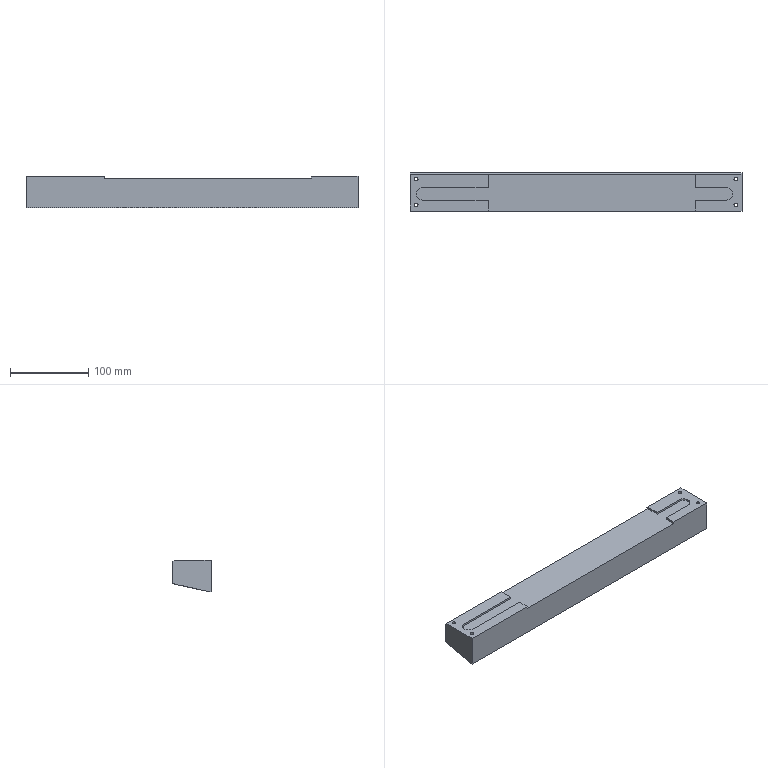Part | 2 solids | 43 faces | box 425 x 49 x 40 mm | volume 688299 mm3 | plane 27 | cylinder 14 | cone 2 | commonest cylinder face diameters 4.5 x4 8 x4 3.242 x2 16 x2 41 x2
STEP:
#1=CARTESIAN_POINT('',(206.75,-16.5,0.));
#2=VERTEX_POINT('',#1);
#3=CARTESIAN_POINT('',(204.5,-16.5,0.));
#4=DIRECTION('',(0.,0.,1.));
#5=DIRECTION('',(1.,0.,0.));
#6=AXIS2_PLACEMENT_3D('',#3,#4,#5);
#7=CIRCLE('',#6,2.25);
#8=EDGE_CURVE('',#2,#2,#7,.T.);
#9=ORIENTED_EDGE('',*,*,#8,.T.);
#10=EDGE_LOOP('',(#9));
#11=FACE_BOUND('',#10,.T.);
#12=CARTESIAN_POINT('',(206.75,-16.5,-5.));
#13=VERTEX_POINT('',#12);
#14=CARTESIAN_POINT('',(204.5,-16.5,-5.));
#15=DIRECTION('',(0.,0.,1.));
#16=DIRECTION('',(1.,0.,0.));
#17=AXIS2_PLACEMENT_3D('',#14,#15,#16);
#18=CIRCLE('',#17,2.25);
#19=EDGE_CURVE('',#13,#13,#18,.T.);
#20=ORIENTED_EDGE('',*,*,#19,.F.);
#21=EDGE_LOOP('',(#20));
#22=FACE_BOUND('',#21,.T.);
#23=CARTESIAN_POINT('',(204.5,-16.5,-40.));
#24=DIRECTION('',(0.,0.,1.));
#25=DIRECTION('',(1.,0.,0.));
#26=AXIS2_PLACEMENT_3D('',#23,#24,#25);
#27=CYLINDRICAL_SURFACE('',#26,2.25);
#28=ADVANCED_FACE('',(#11,#22),#27,.F.);
#29=CARTESIAN_POINT('',(208.5,-16.5,-5.));
#30=VERTEX_POINT('',#29);
#31=CARTESIAN_POINT('',(204.5,-16.5,-5.));
#32=DIRECTION('',(0.,0.,1.));
#33=DIRECTION('',(1.,0.,0.));
#34=AXIS2_PLACEMENT_3D('',#31,#32,#33);
#35=CIRCLE('',#34,4.);
#36=EDGE_CURVE('',#30,#30,#35,.T.);
#37=ORIENTED_EDGE('',*,*,#36,.T.);
#38=EDGE_LOOP('',(#37));
#39=FACE_BOUND('',#38,.T.);
#40=CARTESIAN_POINT('',(200.5,-16.5,-38.895));
#41=VERTEX_POINT('',#40);
#42=CARTESIAN_POINT('',(208.5,-16.5,-38.895));
#43=VERTEX_POINT('',#42);
#44=CARTESIAN_POINT('',(200.5,-16.5,-38.895));
#45=CARTESIAN_POINT('',(200.5,-16.851,-38.973));
#46=CARTESIAN_POINT('',(200.539,-17.202,-39.05));
#47=CARTESIAN_POINT('',(200.616,-17.548,-39.127));
#48=CARTESIAN_POINT('',(200.857,-18.254,-39.283));
#49=CARTESIAN_POINT('',(201.257,-18.891,-39.423));
#50=CARTESIAN_POINT('',(201.508,-19.199,-39.491));
#51=CARTESIAN_POINT('',(202.077,-19.742,-39.612));
#52=CARTESIAN_POINT('',(202.764,-20.135,-39.698));
#53=CARTESIAN_POINT('',(203.126,-20.287,-39.732));
#54=CARTESIAN_POINT('',(203.879,-20.499,-39.779));
#55=CARTESIAN_POINT('',(204.661,-20.525,-39.785));
#56=CARTESIAN_POINT('',(205.049,-20.49,-39.777));
#57=CARTESIAN_POINT('',(205.877,-20.314,-39.738));
#58=CARTESIAN_POINT('',(206.63,-19.931,-39.653));
#59=CARTESIAN_POINT('',(207.005,-19.668,-39.595));
#60=CARTESIAN_POINT('',(207.674,-19.039,-39.456));
#61=CARTESIAN_POINT('',(208.139,-18.253,-39.282));
#62=CARTESIAN_POINT('',(208.316,-17.825,-39.188));
#63=CARTESIAN_POINT('',(208.45,-17.296,-39.071));
#64=CARTESIAN_POINT('',(208.493,-16.757,-38.952));
#65=CARTESIAN_POINT('',(208.498,-16.671,-38.933));
#66=CARTESIAN_POINT('',(208.5,-16.586,-38.914));
#67=CARTESIAN_POINT('',(208.5,-16.5,-38.895));
#68=B_SPLINE_CURVE_WITH_KNOTS('',5,(#44,#45,#46,#47,#48,#49,#50,#51,#52,#53,#54,#55,#56,#57,#58,#59,#60,#61,#62,#63,#64,#65,#66,#67),.UNSPECIFIED.,.F.,.F.,(6,3,3,3,3,3,3,6),(17.986,20.528,23.351,26.114,28.844,32.06,35.352,35.972),.UNSPECIFIED.);
#69=EDGE_CURVE('',#41,#43,#68,.T.);
#70=ORIENTED_EDGE('',*,*,#69,.F.);
#71=CARTESIAN_POINT('',(208.5,-16.5,-38.895));
#72=CARTESIAN_POINT('',(208.5,-16.106,-38.808));
#73=CARTESIAN_POINT('',(208.452,-15.713,-38.721));
#74=CARTESIAN_POINT('',(208.355,-15.326,-38.636));
#75=CARTESIAN_POINT('',(208.069,-14.589,-38.473));
#76=CARTESIAN_POINT('',(207.611,-13.94,-38.329));
#77=CARTESIAN_POINT('',(207.344,-13.646,-38.265));
#78=CARTESIAN_POINT('',(206.748,-13.133,-38.151));
#79=CARTESIAN_POINT('',(206.042,-12.778,-38.073));
#80=CARTESIAN_POINT('',(205.672,-12.645,-38.043));
#81=CARTESIAN_POINT('',(204.91,-12.474,-38.006));
#82=CARTESIAN_POINT('',(204.128,-12.489,-38.009));
#83=CARTESIAN_POINT('',(203.742,-12.544,-38.021));
#84=CARTESIAN_POINT('',(202.925,-12.763,-38.07));
#85=CARTESIAN_POINT('',(202.192,-13.185,-38.163));
#86=CARTESIAN_POINT('',(201.833,-13.468,-38.225));
#87=CARTESIAN_POINT('',(201.197,-14.132,-38.372));
#88=CARTESIAN_POINT('',(200.773,-14.942,-38.551));
#89=CARTESIAN_POINT('',(200.62,-15.379,-38.647));
#90=CARTESIAN_POINT('',(200.522,-15.873,-38.757));
#91=CARTESIAN_POINT('',(200.502,-16.371,-38.867));
#92=CARTESIAN_POINT('',(200.501,-16.414,-38.876));
#93=CARTESIAN_POINT('',(200.5,-16.457,-38.886));
#94=CARTESIAN_POINT('',(200.5,-16.5,-38.895));
#95=B_SPLINE_CURVE_WITH_KNOTS('',5,(#71,#72,#73,#74,#75,#76,#77,#78,#79,#80,#81,#82,#83,#84,#85,#86,#87,#88,#89,#90,#91,#92,#93,#94),.UNSPECIFIED.,.F.,.F.,(6,3,3,3,3,3,3,6),(0.,2.851,5.667,8.426,11.154,14.376,17.675,17.986),.UNSPECIFIED.);
#96=EDGE_CURVE('',#43,#41,#95,.T.);
#97=ORIENTED_EDGE('',*,*,#96,.F.);
#98=EDGE_LOOP('',(#70,#97));
#99=FACE_BOUND('',#98,.T.);
#100=CARTESIAN_POINT('',(204.5,-16.5,-40.));
#101=DIRECTION('',(0.,0.,1.));
#102=DIRECTION('',(1.,0.,0.));
#103=AXIS2_PLACEMENT_3D('',#100,#101,#102);
#104=CYLINDRICAL_SURFACE('',#103,4.);
#105=ADVANCED_FACE('',(#39,#99),#104,.F.);
#106=ORIENTED_EDGE('',*,*,#19,.T.);
#107=EDGE_LOOP('',(#106));
#108=FACE_BOUND('',#107,.T.);
#109=ORIENTED_EDGE('',*,*,#36,.F.);
#110=EDGE_LOOP('',(#109));
#111=FACE_BOUND('',#110,.T.);
#112=CARTESIAN_POINT('',(-202.25,-16.5,-5.));
#113=DIRECTION('',(0.,0.,1.));
#114=DIRECTION('',(1.,0.,0.));
#115=AXIS2_PLACEMENT_3D('',#112,#113,#114);
#116=PLANE('',#115);
#117=ADVANCED_FACE('',(#108,#111),#116,.F.);
#118=CARTESIAN_POINT('',(206.75,16.5,0.));
#119=VERTEX_POINT('',#118);
#120=CARTESIAN_POINT('',(204.5,16.5,0.));
#121=DIRECTION('',(0.,0.,1.));
#122=DIRECTION('',(1.,0.,0.));
#123=AXIS2_PLACEMENT_3D('',#120,#121,#122);
#124=CIRCLE('',#123,2.25);
#125=EDGE_CURVE('',#119,#119,#124,.T.);
#126=ORIENTED_EDGE('',*,*,#125,.T.);
#127=EDGE_LOOP('',(#126));
#128=FACE_BOUND('',#127,.T.);
#129=CARTESIAN_POINT('',(206.75,16.5,-5.));
#130=VERTEX_POINT('',#129);
#131=CARTESIAN_POINT('',(204.5,16.5,-5.));
#132=DIRECTION('',(0.,0.,1.));
#133=DIRECTION('',(1.,0.,0.));
#134=AXIS2_PLACEMENT_3D('',#131,#132,#133);
#135=CIRCLE('',#134,2.25);
#136=EDGE_CURVE('',#130,#130,#135,.T.);
#137=ORIENTED_EDGE('',*,*,#136,.F.);
#138=EDGE_LOOP('',(#137));
#139=FACE_BOUND('',#138,.T.);
#140=CARTESIAN_POINT('',(204.5,16.5,-40.));
#141=DIRECTION('',(0.,0.,1.));
#142=DIRECTION('',(1.,0.,0.));
#143=AXIS2_PLACEMENT_3D('',#140,#141,#142);
#144=CYLINDRICAL_SURFACE('',#143,2.25);
#145=ADVANCED_FACE('',(#128,#139),#144,.F.);
#146=CARTESIAN_POINT('',(208.5,16.5,-5.));
#147=VERTEX_POINT('',#146);
#148=CARTESIAN_POINT('',(204.5,16.5,-5.));
#149=DIRECTION('',(0.,0.,1.));
#150=DIRECTION('',(1.,0.,0.));
#151=AXIS2_PLACEMENT_3D('',#148,#149,#150);
#152=CIRCLE('',#151,4.);
#153=EDGE_CURVE('',#147,#147,#152,.T.);
#154=ORIENTED_EDGE('',*,*,#153,.T.);
#155=EDGE_LOOP('',(#154));
#156=FACE_BOUND('',#155,.T.);
#157=CARTESIAN_POINT('',(200.5,16.5,-31.603));
#158=VERTEX_POINT('',#157);
#159=CARTESIAN_POINT('',(208.5,16.5,-31.603));
#160=VERTEX_POINT('',#159);
#161=CARTESIAN_POINT('',(200.5,16.5,-31.603));
#162=CARTESIAN_POINT('',(200.5,16.149,-31.681));
#163=CARTESIAN_POINT('',(200.539,15.798,-31.759));
#164=CARTESIAN_POINT('',(200.616,15.452,-31.835));
#165=CARTESIAN_POINT('',(200.857,14.746,-31.991));
#166=CARTESIAN_POINT('',(201.257,14.109,-32.132));
#167=CARTESIAN_POINT('',(201.508,13.801,-32.2));
#168=CARTESIAN_POINT('',(202.077,13.258,-32.32));
#169=CARTESIAN_POINT('',(202.764,12.865,-32.407));
#170=CARTESIAN_POINT('',(203.126,12.713,-32.44));
#171=CARTESIAN_POINT('',(203.879,12.501,-32.487));
#172=CARTESIAN_POINT('',(204.661,12.475,-32.493));
#173=CARTESIAN_POINT('',(205.049,12.51,-32.485));
#174=CARTESIAN_POINT('',(205.877,12.686,-32.446));
#175=CARTESIAN_POINT('',(206.63,13.069,-32.362));
#176=CARTESIAN_POINT('',(207.005,13.332,-32.303));
#177=CARTESIAN_POINT('',(207.674,13.961,-32.164));
#178=CARTESIAN_POINT('',(208.139,14.747,-31.991));
#179=CARTESIAN_POINT('',(208.316,15.175,-31.896));
#180=CARTESIAN_POINT('',(208.45,15.704,-31.779));
#181=CARTESIAN_POINT('',(208.493,16.243,-31.66));
#182=CARTESIAN_POINT('',(208.498,16.329,-31.641));
#183=CARTESIAN_POINT('',(208.5,16.414,-31.622));
#184=CARTESIAN_POINT('',(208.5,16.5,-31.603));
#185=B_SPLINE_CURVE_WITH_KNOTS('',5,(#161,#162,#163,#164,#165,#166,#167,#168,#169,#170,#171,#172,#173,#174,#175,#176,#177,#178,#179,#180,#181,#182,#183,#184),.UNSPECIFIED.,.F.,.F.,(6,3,3,3,3,3,3,6),(17.986,20.528,23.351,26.114,28.844,32.06,35.352,35.972),.UNSPECIFIED.);
#186=EDGE_CURVE('',#158,#160,#185,.T.);
#187=ORIENTED_EDGE('',*,*,#186,.F.);
#188=CARTESIAN_POINT('',(208.5,16.5,-31.603));
#189=CARTESIAN_POINT('',(208.5,16.894,-31.516));
#190=CARTESIAN_POINT('',(208.452,17.287,-31.429));
#191=CARTESIAN_POINT('',(208.355,17.674,-31.344));
#192=CARTESIAN_POINT('',(208.069,18.411,-31.181));
#193=CARTESIAN_POINT('',(207.611,19.06,-31.038));
#194=CARTESIAN_POINT('',(207.344,19.354,-30.973));
#195=CARTESIAN_POINT('',(206.748,19.867,-30.86));
#196=CARTESIAN_POINT('',(206.042,20.222,-30.781));
#197=CARTESIAN_POINT('',(205.672,20.355,-30.752));
#198=CARTESIAN_POINT('',(204.91,20.526,-30.714));
#199=CARTESIAN_POINT('',(204.128,20.511,-30.717));
#200=CARTESIAN_POINT('',(203.742,20.456,-30.729));
#201=CARTESIAN_POINT('',(202.925,20.237,-30.778));
#202=CARTESIAN_POINT('',(202.192,19.815,-30.871));
#203=CARTESIAN_POINT('',(201.833,19.532,-30.933));
#204=CARTESIAN_POINT('',(201.197,18.868,-31.08));
#205=CARTESIAN_POINT('',(200.773,18.058,-31.259));
#206=CARTESIAN_POINT('',(200.62,17.621,-31.356));
#207=CARTESIAN_POINT('',(200.522,17.127,-31.465));
#208=CARTESIAN_POINT('',(200.502,16.629,-31.575));
#209=CARTESIAN_POINT('',(200.501,16.586,-31.584));
#210=CARTESIAN_POINT('',(200.5,16.543,-31.594));
#211=CARTESIAN_POINT('',(200.5,16.5,-31.603));
#212=B_SPLINE_CURVE_WITH_KNOTS('',5,(#188,#189,#190,#191,#192,#193,#194,#195,#196,#197,#198,#199,#200,#201,#202,#203,#204,#205,#206,#207,#208,#209,#210,#211),.UNSPECIFIED.,.F.,.F.,(6,3,3,3,3,3,3,6),(0.,2.851,5.667,8.426,11.154,14.376,17.675,17.986),.UNSPECIFIED.);
#213=EDGE_CURVE('',#160,#158,#212,.T.);
#214=ORIENTED_EDGE('',*,*,#213,.F.);
#215=EDGE_LOOP('',(#187,#214));
#216=FACE_BOUND('',#215,.T.);
#217=CARTESIAN_POINT('',(204.5,16.5,-40.));
#218=DIRECTION('',(0.,0.,1.));
#219=DIRECTION('',(1.,0.,0.));
#220=AXIS2_PLACEMENT_3D('',#217,#218,#219);
#221=CYLINDRICAL_SURFACE('',#220,4.);
#222=ADVANCED_FACE('',(#156,#216),#221,.F.);
#223=ORIENTED_EDGE('',*,*,#136,.T.);
#224=EDGE_LOOP('',(#223));
#225=FACE_BOUND('',#224,.T.);
#226=ORIENTED_EDGE('',*,*,#153,.F.);
#227=EDGE_LOOP('',(#226));
#228=FACE_BOUND('',#227,.T.);
#229=CARTESIAN_POINT('',(-202.25,-16.5,-5.));
#230=DIRECTION('',(0.,0.,1.));
#231=DIRECTION('',(1.,0.,0.));
#232=AXIS2_PLACEMENT_3D('',#229,#230,#231);
#233=PLANE('',#232);
#234=ADVANCED_FACE('',(#225,#228),#233,.F.);
#235=CARTESIAN_POINT('',(-202.25,16.5,0.));
#236=VERTEX_POINT('',#235);
#237=CARTESIAN_POINT('',(-204.5,16.5,0.));
#238=DIRECTION('',(0.,0.,1.));
#239=DIRECTION('',(1.,0.,0.));
#240=AXIS2_PLACEMENT_3D('',#237,#238,#239);
#241=CIRCLE('',#240,2.25);
#242=EDGE_CURVE('',#236,#236,#241,.T.);
#243=ORIENTED_EDGE('',*,*,#242,.T.);
#244=EDGE_LOOP('',(#243));
#245=FACE_BOUND('',#244,.T.);
#246=CARTESIAN_POINT('',(-202.25,16.5,-5.));
#247=VERTEX_POINT('',#246);
#248=CARTESIAN_POINT('',(-204.5,16.5,-5.));
#249=DIRECTION('',(0.,0.,1.));
#250=DIRECTION('',(1.,0.,0.));
#251=AXIS2_PLACEMENT_3D('',#248,#249,#250);
#252=CIRCLE('',#251,2.25);
#253=EDGE_CURVE('',#247,#247,#252,.T.);
#254=ORIENTED_EDGE('',*,*,#253,.F.);
#255=EDGE_LOOP('',(#254));
#256=FACE_BOUND('',#255,.T.);
#257=CARTESIAN_POINT('',(-204.5,16.5,-40.));
#258=DIRECTION('',(0.,0.,1.));
#259=DIRECTION('',(1.,0.,0.));
#260=AXIS2_PLACEMENT_3D('',#257,#258,#259);
#261=CYLINDRICAL_SURFACE('',#260,2.25);
#262=ADVANCED_FACE('',(#245,#256),#261,.F.);
#263=CARTESIAN_POINT('',(-200.5,16.5,-5.));
#264=VERTEX_POINT('',#263);
#265=CARTESIAN_POINT('',(-204.5,16.5,-5.));
#266=DIRECTION('',(0.,0.,1.));
#267=DIRECTION('',(1.,0.,0.));
#268=AXIS2_PLACEMENT_3D('',#265,#266,#267);
#269=CIRCLE('',#268,4.);
#270=EDGE_CURVE('',#264,#264,#269,.T.);
#271=ORIENTED_EDGE('',*,*,#270,.T.);
#272=EDGE_LOOP('',(#271));
#273=FACE_BOUND('',#272,.T.);
#274=CARTESIAN_POINT('',(-208.5,16.5,-31.603));
#275=VERTEX_POINT('',#274);
#276=CARTESIAN_POINT('',(-200.5,16.5,-31.603));
#277=VERTEX_POINT('',#276);
#278=CARTESIAN_POINT('',(-208.5,16.5,-31.603));
#279=CARTESIAN_POINT('',(-208.5,16.149,-31.681));
#280=CARTESIAN_POINT('',(-208.461,15.798,-31.759));
#281=CARTESIAN_POINT('',(-208.384,15.452,-31.835));
#282=CARTESIAN_POINT('',(-208.143,14.746,-31.991));
#283=CARTESIAN_POINT('',(-207.743,14.109,-32.132));
#284=CARTESIAN_POINT('',(-207.492,13.801,-32.2));
#285=CARTESIAN_POINT('',(-206.923,13.258,-32.32));
#286=CARTESIAN_POINT('',(-206.236,12.865,-32.407));
#287=CARTESIAN_POINT('',(-205.874,12.713,-32.44));
#288=CARTESIAN_POINT('',(-205.121,12.501,-32.487));
#289=CARTESIAN_POINT('',(-204.339,12.475,-32.493));
#290=CARTESIAN_POINT('',(-203.951,12.51,-32.485));
#291=CARTESIAN_POINT('',(-203.123,12.686,-32.446));
#292=CARTESIAN_POINT('',(-202.37,13.069,-32.362));
#293=CARTESIAN_POINT('',(-201.995,13.332,-32.303));
#294=CARTESIAN_POINT('',(-201.326,13.961,-32.164));
#295=CARTESIAN_POINT('',(-200.861,14.747,-31.991));
#296=CARTESIAN_POINT('',(-200.684,15.175,-31.896));
#297=CARTESIAN_POINT('',(-200.55,15.704,-31.779));
#298=CARTESIAN_POINT('',(-200.507,16.243,-31.66));
#299=CARTESIAN_POINT('',(-200.502,16.329,-31.641));
#300=CARTESIAN_POINT('',(-200.5,16.414,-31.622));
#301=CARTESIAN_POINT('',(-200.5,16.5,-31.603));
#302=B_SPLINE_CURVE_WITH_KNOTS('',5,(#278,#279,#280,#281,#282,#283,#284,#285,#286,#287,#288,#289,#290,#291,#292,#293,#294,#295,#296,#297,#298,#299,#300,#301),.UNSPECIFIED.,.F.,.F.,(6,3,3,3,3,3,3,6),(17.986,20.528,23.351,26.114,28.844,32.06,35.352,35.972),.UNSPECIFIED.);
#303=EDGE_CURVE('',#275,#277,#302,.T.);
#304=ORIENTED_EDGE('',*,*,#303,.F.);
#305=CARTESIAN_POINT('',(-200.5,16.5,-31.603));
#306=CARTESIAN_POINT('',(-200.5,16.894,-31.516));
#307=CARTESIAN_POINT('',(-200.548,17.287,-31.429));
#308=CARTESIAN_POINT('',(-200.645,17.674,-31.344));
#309=CARTESIAN_POINT('',(-200.931,18.411,-31.181));
#310=CARTESIAN_POINT('',(-201.389,19.06,-31.038));
#311=CARTESIAN_POINT('',(-201.656,19.354,-30.973));
#312=CARTESIAN_POINT('',(-202.252,19.867,-30.86));
#313=CARTESIAN_POINT('',(-202.958,20.222,-30.781));
#314=CARTESIAN_POINT('',(-203.328,20.355,-30.752));
#315=CARTESIAN_POINT('',(-204.09,20.526,-30.714));
#316=CARTESIAN_POINT('',(-204.872,20.511,-30.717));
#317=CARTESIAN_POINT('',(-205.258,20.456,-30.729));
#318=CARTESIAN_POINT('',(-206.075,20.237,-30.778));
#319=CARTESIAN_POINT('',(-206.808,19.815,-30.871));
#320=CARTESIAN_POINT('',(-207.167,19.532,-30.933));
#321=CARTESIAN_POINT('',(-207.803,18.868,-31.08));
#322=CARTESIAN_POINT('',(-208.227,18.058,-31.259));
#323=CARTESIAN_POINT('',(-208.38,17.621,-31.356));
#324=CARTESIAN_POINT('',(-208.478,17.127,-31.465));
#325=CARTESIAN_POINT('',(-208.498,16.629,-31.575));
#326=CARTESIAN_POINT('',(-208.499,16.586,-31.584));
#327=CARTESIAN_POINT('',(-208.5,16.543,-31.594));
#328=CARTESIAN_POINT('',(-208.5,16.5,-31.603));
#329=B_SPLINE_CURVE_WITH_KNOTS('',5,(#305,#306,#307,#308,#309,#310,#311,#312,#313,#314,#315,#316,#317,#318,#319,#320,#321,#322,#323,#324,#325,#326,#327,#328),.UNSPECIFIED.,.F.,.F.,(6,3,3,3,3,3,3,6),(0.,2.851,5.667,8.426,11.154,14.376,17.675,17.986),.UNSPECIFIED.);
#330=EDGE_CURVE('',#277,#275,#329,.T.);
#331=ORIENTED_EDGE('',*,*,#330,.F.);
#332=EDGE_LOOP('',(#304,#331));
#333=FACE_BOUND('',#332,.T.);
#334=CARTESIAN_POINT('',(-204.5,16.5,-40.));
#335=DIRECTION('',(0.,0.,1.));
#336=DIRECTION('',(1.,0.,0.));
#337=AXIS2_PLACEMENT_3D('',#334,#335,#336);
#338=CYLINDRICAL_SURFACE('',#337,4.);
#339=ADVANCED_FACE('',(#273,#333),#338,.F.);
#340=ORIENTED_EDGE('',*,*,#253,.T.);
#341=EDGE_LOOP('',(#340));
#342=FACE_BOUND('',#341,.T.);
#343=ORIENTED_EDGE('',*,*,#270,.F.);
#344=EDGE_LOOP('',(#343));
#345=FACE_BOUND('',#344,.T.);
#346=CARTESIAN_POINT('',(-202.25,-16.5,-5.));
#347=DIRECTION('',(0.,0.,1.));
#348=DIRECTION('',(1.,0.,0.));
#349=AXIS2_PLACEMENT_3D('',#346,#347,#348);
#350=PLANE('',#349);
#351=ADVANCED_FACE('',(#342,#345),#350,.F.);
#352=CARTESIAN_POINT('',(-200.5,-16.5,-5.));
#353=VERTEX_POINT('',#352);
#354=CARTESIAN_POINT('',(-204.5,-16.5,-5.));
#355=DIRECTION('',(0.,0.,1.));
#356=DIRECTION('',(1.,0.,0.));
#357=AXIS2_PLACEMENT_3D('',#354,#355,#356);
#358=CIRCLE('',#357,4.);
#359=EDGE_CURVE('',#353,#353,#358,.T.);
#360=ORIENTED_EDGE('',*,*,#359,.T.);
#361=EDGE_LOOP('',(#360));
#362=FACE_BOUND('',#361,.T.);
#363=CARTESIAN_POINT('',(-200.5,-16.5,-38.895));
#364=VERTEX_POINT('',#363);
#365=CARTESIAN_POINT('',(-208.5,-16.5,-38.895));
#366=VERTEX_POINT('',#365);
#367=CARTESIAN_POINT('',(-200.5,-16.5,-38.895));
#368=CARTESIAN_POINT('',(-200.5,-16.106,-38.808));
#369=CARTESIAN_POINT('',(-200.548,-15.713,-38.721));
#370=CARTESIAN_POINT('',(-200.645,-15.326,-38.636));
#371=CARTESIAN_POINT('',(-200.931,-14.589,-38.473));
#372=CARTESIAN_POINT('',(-201.389,-13.94,-38.329));
#373=CARTESIAN_POINT('',(-201.656,-13.646,-38.265));
#374=CARTESIAN_POINT('',(-202.252,-13.133,-38.151));
#375=CARTESIAN_POINT('',(-202.958,-12.778,-38.073));
#376=CARTESIAN_POINT('',(-203.328,-12.645,-38.043));
#377=CARTESIAN_POINT('',(-204.09,-12.474,-38.006));
#378=CARTESIAN_POINT('',(-204.872,-12.489,-38.009));
#379=CARTESIAN_POINT('',(-205.258,-12.544,-38.021));
#380=CARTESIAN_POINT('',(-206.075,-12.763,-38.07));
#381=CARTESIAN_POINT('',(-206.808,-13.185,-38.163));
#382=CARTESIAN_POINT('',(-207.167,-13.468,-38.225));
#383=CARTESIAN_POINT('',(-207.803,-14.132,-38.372));
#384=CARTESIAN_POINT('',(-208.227,-14.942,-38.551));
#385=CARTESIAN_POINT('',(-208.38,-15.379,-38.647));
#386=CARTESIAN_POINT('',(-208.478,-15.873,-38.757));
#387=CARTESIAN_POINT('',(-208.498,-16.371,-38.867));
#388=CARTESIAN_POINT('',(-208.499,-16.414,-38.876));
#389=CARTESIAN_POINT('',(-208.5,-16.457,-38.886));
#390=CARTESIAN_POINT('',(-208.5,-16.5,-38.895));
#391=B_SPLINE_CURVE_WITH_KNOTS('',5,(#367,#368,#369,#370,#371,#372,#373,#374,#375,#376,#377,#378,#379,#380,#381,#382,#383,#384,#385,#386,#387,#388,#389,#390),.UNSPECIFIED.,.F.,.F.,(6,3,3,3,3,3,3,6),(0.,2.851,5.667,8.426,11.154,14.376,17.675,17.986),.UNSPECIFIED.);
#392=EDGE_CURVE('',#364,#366,#391,.T.);
#393=ORIENTED_EDGE('',*,*,#392,.F.);
#394=CARTESIAN_POINT('',(-208.5,-16.5,-38.895));
#395=CARTESIAN_POINT('',(-208.5,-16.851,-38.973));
#396=CARTESIAN_POINT('',(-208.461,-17.202,-39.05));
#397=CARTESIAN_POINT('',(-208.384,-17.548,-39.127));
#398=CARTESIAN_POINT('',(-208.143,-18.254,-39.283));
#399=CARTESIAN_POINT('',(-207.743,-18.891,-39.423));
#400=CARTESIAN_POINT('',(-207.492,-19.199,-39.491));
#401=CARTESIAN_POINT('',(-206.923,-19.742,-39.612));
#402=CARTESIAN_POINT('',(-206.236,-20.135,-39.698));
#403=CARTESIAN_POINT('',(-205.874,-20.287,-39.732));
#404=CARTESIAN_POINT('',(-205.121,-20.499,-39.779));
#405=CARTESIAN_POINT('',(-204.339,-20.525,-39.785));
#406=CARTESIAN_POINT('',(-203.951,-20.49,-39.777));
#407=CARTESIAN_POINT('',(-203.123,-20.314,-39.738));
#408=CARTESIAN_POINT('',(-202.37,-19.931,-39.653));
#409=CARTESIAN_POINT('',(-201.995,-19.668,-39.595));
#410=CARTESIAN_POINT('',(-201.326,-19.039,-39.456));
#411=CARTESIAN_POINT('',(-200.861,-18.253,-39.282));
#412=CARTESIAN_POINT('',(-200.684,-17.825,-39.188));
#413=CARTESIAN_POINT('',(-200.55,-17.296,-39.071));
#414=CARTESIAN_POINT('',(-200.507,-16.757,-38.952));
#415=CARTESIAN_POINT('',(-200.502,-16.671,-38.933));
#416=CARTESIAN_POINT('',(-200.5,-16.586,-38.914));
#417=CARTESIAN_POINT('',(-200.5,-16.5,-38.895));
#418=B_SPLINE_CURVE_WITH_KNOTS('',5,(#394,#395,#396,#397,#398,#399,#400,#401,#402,#403,#404,#405,#406,#407,#408,#409,#410,#411,#412,#413,#414,#415,#416,#417),.UNSPECIFIED.,.F.,.F.,(6,3,3,3,3,3,3,6),(17.986,20.528,23.351,26.114,28.844,32.06,35.352,35.972),.UNSPECIFIED.);
#419=EDGE_CURVE('',#366,#364,#418,.T.);
#420=ORIENTED_EDGE('',*,*,#419,.F.);
#421=EDGE_LOOP('',(#393,#420));
#422=FACE_BOUND('',#421,.T.);
#423=CARTESIAN_POINT('',(-204.5,-16.5,-40.));
#424=DIRECTION('',(0.,0.,1.));
#425=DIRECTION('',(1.,0.,0.));
#426=AXIS2_PLACEMENT_3D('',#423,#424,#425);
#427=CYLINDRICAL_SURFACE('',#426,4.);
#428=ADVANCED_FACE('',(#362,#422),#427,.F.);
#429=CARTESIAN_POINT('',(-112.5,-24.5,0.));
#430=VERTEX_POINT('',#429);
#431=CARTESIAN_POINT('',(-212.5,-24.5,0.));
#432=VERTEX_POINT('',#431);
#433=CARTESIAN_POINT('',(-162.5,-24.5,0.));
#434=DIRECTION('',(-1.,0.,0.));
#435=VECTOR('',#434,1000.);
#436=LINE('',#433,#435);
#437=EDGE_CURVE('',#430,#432,#436,.T.);
#438=ORIENTED_EDGE('',*,*,#437,.T.);
#439=CARTESIAN_POINT('',(-212.5,-24.5,-40.));
#440=VERTEX_POINT('',#439);
#441=CARTESIAN_POINT('',(-212.5,-24.5,-20.));
#442=DIRECTION('',(0.,0.,1.));
#443=VECTOR('',#442,1000.);
#444=LINE('',#441,#443);
#445=EDGE_CURVE('',#440,#432,#444,.T.);
#446=ORIENTED_EDGE('',*,*,#445,.F.);
#447=CARTESIAN_POINT('',(212.5,-24.5,-40.));
#448=VERTEX_POINT('',#447);
#449=CARTESIAN_POINT('',(0.,-24.5,-40.));
#450=DIRECTION('',(1.,0.,0.));
#451=VECTOR('',#450,1000.);
#452=LINE('',#449,#451);
#453=EDGE_CURVE('',#440,#448,#452,.T.);
#454=ORIENTED_EDGE('',*,*,#453,.T.);
#455=CARTESIAN_POINT('',(212.5,-24.5,0.));
#456=VERTEX_POINT('',#455);
#457=CARTESIAN_POINT('',(212.5,-24.5,-20.));
#458=DIRECTION('',(0.,0.,-1.));
#459=VECTOR('',#458,1000.);
#460=LINE('',#457,#459);
#461=EDGE_CURVE('',#456,#448,#460,.T.);
#462=ORIENTED_EDGE('',*,*,#461,.F.);
#463=CARTESIAN_POINT('',(152.5,-24.5,0.));
#464=VERTEX_POINT('',#463);
#465=CARTESIAN_POINT('',(182.5,-24.5,0.));
#466=DIRECTION('',(-1.,0.,0.));
#467=VECTOR('',#466,1000.);
#468=LINE('',#465,#467);
#469=EDGE_CURVE('',#456,#464,#468,.T.);
#470=ORIENTED_EDGE('',*,*,#469,.T.);
#471=CARTESIAN_POINT('',(152.5,-24.5,-2.5));
#472=VERTEX_POINT('',#471);
#473=CARTESIAN_POINT('',(152.5,-24.5,-1.25));
#474=DIRECTION('',(0.,0.,-1.));
#475=VECTOR('',#474,1000.);
#476=LINE('',#473,#475);
#477=EDGE_CURVE('',#464,#472,#476,.T.);
#478=ORIENTED_EDGE('',*,*,#477,.T.);
#479=CARTESIAN_POINT('',(-112.5,-24.5,-2.5));
#480=VERTEX_POINT('',#479);
#481=CARTESIAN_POINT('',(20.,-24.5,-2.5));
#482=DIRECTION('',(1.,0.,0.));
#483=VECTOR('',#482,1000.);
#484=LINE('',#481,#483);
#485=EDGE_CURVE('',#480,#472,#484,.T.);
#486=ORIENTED_EDGE('',*,*,#485,.F.);
#487=CARTESIAN_POINT('',(-112.5,-24.5,-1.25));
#488=DIRECTION('',(0.,0.,-1.));
#489=VECTOR('',#488,1000.);
#490=LINE('',#487,#489);
#491=EDGE_CURVE('',#430,#480,#490,.T.);
#492=ORIENTED_EDGE('',*,*,#491,.F.);
#493=EDGE_LOOP('',(#438,#446,#454,#462,#470,#478,#486,#492));
#494=FACE_BOUND('',#493,.T.);
#495=CARTESIAN_POINT('',(-212.5,-24.5,0.));
#496=DIRECTION('',(0.,-1.,0.));
#497=DIRECTION('',(1.,0.,0.));
#498=AXIS2_PLACEMENT_3D('',#495,#496,#497);
#499=PLANE('',#498);
#500=ADVANCED_FACE('',(#494),#499,.T.);
#501=ORIENTED_EDGE('',*,*,#491,.T.);
#502=CARTESIAN_POINT('',(-112.5,-10.5,-2.5));
#503=VERTEX_POINT('',#502);
#504=CARTESIAN_POINT('',(-112.5,-17.5,-2.5));
#505=DIRECTION('',(0.,1.,0.));
#506=VECTOR('',#505,1000.);
#507=LINE('',#504,#506);
#508=EDGE_CURVE('',#480,#503,#507,.T.);
#509=ORIENTED_EDGE('',*,*,#508,.T.);
#510=CARTESIAN_POINT('',(-112.5,-10.5,0.));
#511=VERTEX_POINT('',#510);
#512=CARTESIAN_POINT('',(-112.5,-10.5,-1.25));
#513=DIRECTION('',(0.,0.,-1.));
#514=VECTOR('',#513,1000.);
#515=LINE('',#512,#514);
#516=EDGE_CURVE('',#511,#503,#515,.T.);
#517=ORIENTED_EDGE('',*,*,#516,.F.);
#518=CARTESIAN_POINT('',(-112.5,-17.5,0.));
#519=DIRECTION('',(0.,1.,0.));
#520=VECTOR('',#519,1000.);
#521=LINE('',#518,#520);
#522=EDGE_CURVE('',#430,#511,#521,.T.);
#523=ORIENTED_EDGE('',*,*,#522,.F.);
#524=EDGE_LOOP('',(#501,#509,#517,#523));
#525=FACE_BOUND('',#524,.T.);
#526=CARTESIAN_POINT('',(-112.5,5.5,0.));
#527=DIRECTION('',(-1.,0.,0.));
#528=DIRECTION('',(0.,1.,0.));
#529=AXIS2_PLACEMENT_3D('',#526,#527,#528);
#530=PLANE('',#529);
#531=ADVANCED_FACE('',(#525),#530,.F.);
#532=CARTESIAN_POINT('',(-196.5,-10.5,-2.5));
#533=VERTEX_POINT('',#532);
#534=CARTESIAN_POINT('',(-196.5,-10.5,0.));
#535=VERTEX_POINT('',#534);
#536=CARTESIAN_POINT('',(-196.5,-10.5,-1.25));
#537=DIRECTION('',(0.,0.,1.));
#538=VECTOR('',#537,1000.);
#539=LINE('',#536,#538);
#540=EDGE_CURVE('',#533,#535,#539,.T.);
#541=ORIENTED_EDGE('',*,*,#540,.T.);
#542=CARTESIAN_POINT('',(-154.5,-10.5,0.));
#543=DIRECTION('',(-1.,0.,0.));
#544=VECTOR('',#543,1000.);
#545=LINE('',#542,#544);
#546=EDGE_CURVE('',#511,#535,#545,.T.);
#547=ORIENTED_EDGE('',*,*,#546,.F.);
#548=ORIENTED_EDGE('',*,*,#516,.T.);
#549=CARTESIAN_POINT('',(-154.5,-10.5,-2.5));
#550=DIRECTION('',(-1.,0.,0.));
#551=VECTOR('',#550,1000.);
#552=LINE('',#549,#551);
#553=EDGE_CURVE('',#503,#533,#552,.T.);
#554=ORIENTED_EDGE('',*,*,#553,.T.);
#555=EDGE_LOOP('',(#541,#547,#548,#554));
#556=FACE_BOUND('',#555,.T.);
#557=CARTESIAN_POINT('',(-112.5,-10.5,0.));
#558=DIRECTION('',(0.,-1.,0.));
#559=DIRECTION('',(-1.,0.,0.));
#560=AXIS2_PLACEMENT_3D('',#557,#558,#559);
#561=PLANE('',#560);
#562=ADVANCED_FACE('',(#556),#561,.F.);
#563=CARTESIAN_POINT('',(-196.5,5.5,0.));
#564=VERTEX_POINT('',#563);
#565=CARTESIAN_POINT('',(-196.5,5.5,-2.5));
#566=VERTEX_POINT('',#565);
#567=CARTESIAN_POINT('',(-196.5,5.5,-1.25));
#568=DIRECTION('',(0.,0.,-1.));
#569=VECTOR('',#568,1000.);
#570=LINE('',#567,#569);
#571=EDGE_CURVE('',#564,#566,#570,.T.);
#572=ORIENTED_EDGE('',*,*,#571,.F.);
#573=CARTESIAN_POINT('',(-196.5,-2.5,0.));
#574=DIRECTION('',(0.,0.,1.));
#575=DIRECTION('',(1.,0.,0.));
#576=AXIS2_PLACEMENT_3D('',#573,#574,#575);
#577=CIRCLE('',#576,8.);
#578=EDGE_CURVE('',#564,#535,#577,.T.);
#579=ORIENTED_EDGE('',*,*,#578,.T.);
#580=ORIENTED_EDGE('',*,*,#540,.F.);
#581=CARTESIAN_POINT('',(-196.5,-2.5,-2.5));
#582=DIRECTION('',(0.,0.,1.));
#583=DIRECTION('',(1.,0.,0.));
#584=AXIS2_PLACEMENT_3D('',#581,#582,#583);
#585=CIRCLE('',#584,8.);
#586=EDGE_CURVE('',#566,#533,#585,.T.);
#587=ORIENTED_EDGE('',*,*,#586,.F.);
#588=EDGE_LOOP('',(#572,#579,#580,#587));
#589=FACE_BOUND('',#588,.T.);
#590=CARTESIAN_POINT('',(-196.5,-2.5,-1.25));
#591=DIRECTION('',(0.,0.,1.));
#592=DIRECTION('',(0.,1.,0.));
#593=AXIS2_PLACEMENT_3D('',#590,#591,#592);
#594=CYLINDRICAL_SURFACE('',#593,8.);
#595=ADVANCED_FACE('',(#589),#594,.F.);
#596=CARTESIAN_POINT('',(-112.5,5.5,0.));
#597=VERTEX_POINT('',#596);
#598=CARTESIAN_POINT('',(-112.5,5.5,-2.5));
#599=VERTEX_POINT('',#598);
#600=CARTESIAN_POINT('',(-112.5,5.5,-1.25));
#601=DIRECTION('',(0.,0.,-1.));
#602=VECTOR('',#601,1000.);
#603=LINE('',#600,#602);
#604=EDGE_CURVE('',#597,#599,#603,.T.);
#605=ORIENTED_EDGE('',*,*,#604,.F.);
#606=CARTESIAN_POINT('',(-154.5,5.5,0.));
#607=DIRECTION('',(1.,0.,0.));
#608=VECTOR('',#607,1000.);
#609=LINE('',#606,#608);
#610=EDGE_CURVE('',#564,#597,#609,.T.);
#611=ORIENTED_EDGE('',*,*,#610,.F.);
#612=ORIENTED_EDGE('',*,*,#571,.T.);
#613=CARTESIAN_POINT('',(-154.5,5.5,-2.5));
#614=DIRECTION('',(1.,0.,0.));
#615=VECTOR('',#614,1000.);
#616=LINE('',#613,#615);
#617=EDGE_CURVE('',#566,#599,#616,.T.);
#618=ORIENTED_EDGE('',*,*,#617,.T.);
#619=EDGE_LOOP('',(#605,#611,#612,#618));
#620=FACE_BOUND('',#619,.T.);
#621=CARTESIAN_POINT('',(152.5,5.5,0.));
#622=DIRECTION('',(0.,1.,0.));
#623=DIRECTION('',(1.,0.,0.));
#624=AXIS2_PLACEMENT_3D('',#621,#622,#623);
#625=PLANE('',#624);
#626=ADVANCED_FACE('',(#620),#625,.F.);
#627=CARTESIAN_POINT('',(-112.5,22.5,0.));
#628=VERTEX_POINT('',#627);
#629=CARTESIAN_POINT('',(-112.5,24.5,-2.));
#630=VERTEX_POINT('',#629);
#631=CARTESIAN_POINT('',(-112.5,23.5,-1.));
#632=DIRECTION('',(0.,0.7071,-0.7071));
#633=VECTOR('',#632,1000.);
#634=LINE('',#631,#633);
#635=EDGE_CURVE('',#628,#630,#634,.T.);
#636=ORIENTED_EDGE('',*,*,#635,.F.);
#637=CARTESIAN_POINT('',(-112.5,14.,0.));
#638=DIRECTION('',(0.,1.,0.));
#639=VECTOR('',#638,1000.);
#640=LINE('',#637,#639);
#641=EDGE_CURVE('',#597,#628,#640,.T.);
#642=ORIENTED_EDGE('',*,*,#641,.F.);
#643=ORIENTED_EDGE('',*,*,#604,.T.);
#644=CARTESIAN_POINT('',(-112.5,22.5,-2.5));
#645=VERTEX_POINT('',#644);
#646=CARTESIAN_POINT('',(-112.5,14.,-2.5));
#647=DIRECTION('',(0.,1.,0.));
#648=VECTOR('',#647,1000.);
#649=LINE('',#646,#648);
#650=EDGE_CURVE('',#599,#645,#649,.T.);
#651=ORIENTED_EDGE('',*,*,#650,.T.);
#652=CARTESIAN_POINT('',(-112.5,24.5,-4.5));
#653=VERTEX_POINT('',#652);
#654=CARTESIAN_POINT('',(-112.5,23.5,-3.5));
#655=DIRECTION('',(0.,-0.7071,0.7071));
#656=VECTOR('',#655,1000.);
#657=LINE('',#654,#656);
#658=EDGE_CURVE('',#653,#645,#657,.T.);
#659=ORIENTED_EDGE('',*,*,#658,.F.);
#660=CARTESIAN_POINT('',(-112.5,24.5,-3.25));
#661=DIRECTION('',(0.,0.,1.));
#662=VECTOR('',#661,1000.);
#663=LINE('',#660,#662);
#664=EDGE_CURVE('',#653,#630,#663,.T.);
#665=ORIENTED_EDGE('',*,*,#664,.T.);
#666=EDGE_LOOP('',(#636,#642,#643,#651,#659,#665));
#667=FACE_BOUND('',#666,.T.);
#668=CARTESIAN_POINT('',(-112.5,5.5,0.));
#669=DIRECTION('',(-1.,0.,0.));
#670=DIRECTION('',(0.,1.,0.));
#671=AXIS2_PLACEMENT_3D('',#668,#669,#670);
#672=PLANE('',#671);
#673=ADVANCED_FACE('',(#667),#672,.F.);
#674=ORIENTED_EDGE('',*,*,#635,.T.);
#675=CARTESIAN_POINT('',(-212.5,24.5,-2.));
#676=VERTEX_POINT('',#675);
#677=CARTESIAN_POINT('',(-162.5,24.5,-2.));
#678=DIRECTION('',(1.,0.,0.));
#679=VECTOR('',#678,1000.);
#680=LINE('',#677,#679);
#681=EDGE_CURVE('',#676,#630,#680,.T.);
#682=ORIENTED_EDGE('',*,*,#681,.F.);
#683=CARTESIAN_POINT('',(-212.5,22.5,0.));
#684=VERTEX_POINT('',#683);
#685=CARTESIAN_POINT('',(-212.5,23.5,-1.));
#686=DIRECTION('',(0.,0.7071,-0.7071));
#687=VECTOR('',#686,1000.);
#688=LINE('',#685,#687);
#689=EDGE_CURVE('',#684,#676,#688,.T.);
#690=ORIENTED_EDGE('',*,*,#689,.F.);
#691=CARTESIAN_POINT('',(-162.5,22.5,0.));
#692=DIRECTION('',(1.,0.,0.));
#693=VECTOR('',#692,1000.);
#694=LINE('',#691,#693);
#695=EDGE_CURVE('',#684,#628,#694,.T.);
#696=ORIENTED_EDGE('',*,*,#695,.T.);
#697=EDGE_LOOP('',(#674,#682,#690,#696));
#698=FACE_BOUND('',#697,.T.);
#699=CARTESIAN_POINT('',(0.,22.5,0.));
#700=DIRECTION('',(0.,0.7071,0.7071));
#701=DIRECTION('',(1.,0.,0.));
#702=AXIS2_PLACEMENT_3D('',#699,#700,#701);
#703=PLANE('',#702);
#704=ADVANCED_FACE('',(#698),#703,.T.);
#705=CARTESIAN_POINT('',(-212.5,-21.5,-40.));
#706=VERTEX_POINT('',#705);
#707=CARTESIAN_POINT('',(-212.5,-23.,-40.));
#708=DIRECTION('',(0.,1.,0.));
#709=VECTOR('',#708,1000.);
#710=LINE('',#707,#709);
#711=EDGE_CURVE('',#440,#706,#710,.T.);
#712=ORIENTED_EDGE('',*,*,#711,.T.);
#713=CARTESIAN_POINT('',(212.5,-21.5,-40.));
#714=VERTEX_POINT('',#713);
#715=CARTESIAN_POINT('',(0.,-21.5,-40.));
#716=DIRECTION('',(1.,0.,0.));
#717=VECTOR('',#716,1000.);
#718=LINE('',#715,#717);
#719=EDGE_CURVE('',#706,#714,#718,.T.);
#720=ORIENTED_EDGE('',*,*,#719,.T.);
#721=CARTESIAN_POINT('',(212.5,-23.,-40.));
#722=DIRECTION('',(0.,1.,0.));
#723=VECTOR('',#722,1000.);
#724=LINE('',#721,#723);
#725=EDGE_CURVE('',#448,#714,#724,.T.);
#726=ORIENTED_EDGE('',*,*,#725,.F.);
#727=ORIENTED_EDGE('',*,*,#453,.F.);
#728=EDGE_LOOP('',(#712,#720,#726,#727));
#729=FACE_BOUND('',#728,.T.);
#730=CARTESIAN_POINT('',(-212.5,-28.5,-40.));
#731=DIRECTION('',(0.,0.,-1.));
#732=DIRECTION('',(0.,1.,0.));
#733=AXIS2_PLACEMENT_3D('',#730,#731,#732);
#734=PLANE('',#733);
#735=ADVANCED_FACE('',(#729),#734,.T.);
#736=ORIENTED_EDGE('',*,*,#96,.T.);
#737=ORIENTED_EDGE('',*,*,#69,.T.);
#738=EDGE_LOOP('',(#736,#737));
#739=FACE_BOUND('',#738,.T.);
#740=ORIENTED_EDGE('',*,*,#213,.T.);
#741=ORIENTED_EDGE('',*,*,#186,.T.);
#742=EDGE_LOOP('',(#740,#741));
#743=FACE_BOUND('',#742,.T.);
#744=ORIENTED_EDGE('',*,*,#330,.T.);
#745=ORIENTED_EDGE('',*,*,#303,.T.);
#746=EDGE_LOOP('',(#744,#745));
#747=FACE_BOUND('',#746,.T.);
#748=CARTESIAN_POINT('',(-142.,2.042,-34.798));
#749=VERTEX_POINT('',#748);
#750=CARTESIAN_POINT('',(-162.5,2.042,-34.798));
#751=DIRECTION('',(0.,0.2158,-0.9764));
#752=DIRECTION('',(1.,0.,0.));
#753=AXIS2_PLACEMENT_3D('',#750,#751,#752);
#754=CIRCLE('',#753,20.5);
#755=EDGE_CURVE('',#749,#749,#754,.T.);
#756=ORIENTED_EDGE('',*,*,#755,.F.);
#757=EDGE_LOOP('',(#756));
#758=FACE_BOUND('',#757,.T.);
#759=ORIENTED_EDGE('',*,*,#419,.T.);
#760=ORIENTED_EDGE('',*,*,#392,.T.);
#761=EDGE_LOOP('',(#759,#760));
#762=FACE_BOUND('',#761,.T.);
#763=ORIENTED_EDGE('',*,*,#719,.F.);
#764=CARTESIAN_POINT('',(-212.5,24.5,-29.836));
#765=VERTEX_POINT('',#764);
#766=CARTESIAN_POINT('',(-212.5,1.5,-34.918));
#767=DIRECTION('',(0.,-0.9764,-0.2158));
#768=VECTOR('',#767,1000.);
#769=LINE('',#766,#768);
#770=EDGE_CURVE('',#765,#706,#769,.T.);
#771=ORIENTED_EDGE('',*,*,#770,.F.);
#772=CARTESIAN_POINT('',(212.5,24.5,-29.836));
#773=VERTEX_POINT('',#772);
#774=CARTESIAN_POINT('',(0.,24.5,-29.836));
#775=DIRECTION('',(1.,0.,0.));
#776=VECTOR('',#775,1000.);
#777=LINE('',#774,#776);
#778=EDGE_CURVE('',#765,#773,#777,.T.);
#779=ORIENTED_EDGE('',*,*,#778,.T.);
#780=CARTESIAN_POINT('',(212.5,1.5,-34.918));
#781=DIRECTION('',(0.,-0.9764,-0.2158));
#782=VECTOR('',#781,1000.);
#783=LINE('',#780,#782);
#784=EDGE_CURVE('',#773,#714,#783,.T.);
#785=ORIENTED_EDGE('',*,*,#784,.T.);
#786=EDGE_LOOP('',(#763,#771,#779,#785));
#787=FACE_BOUND('',#786,.T.);
#788=CARTESIAN_POINT('',(-212.5,24.5,-29.836));
#789=DIRECTION('',(0.,-0.2158,0.9764));
#790=DIRECTION('',(0.,-0.9764,-0.2158));
#791=AXIS2_PLACEMENT_3D('',#788,#789,#790);
#792=PLANE('',#791);
#793=ADVANCED_FACE('',(#739,#743,#747,#758,#762,#787),#792,.F.);
#794=ORIENTED_EDGE('',*,*,#664,.F.);
#795=CARTESIAN_POINT('',(152.5,24.5,-4.5));
#796=VERTEX_POINT('',#795);
#797=CARTESIAN_POINT('',(0.,24.5,-4.5));
#798=DIRECTION('',(-1.,0.,0.));
#799=VECTOR('',#798,1000.);
#800=LINE('',#797,#799);
#801=EDGE_CURVE('',#796,#653,#800,.T.);
#802=ORIENTED_EDGE('',*,*,#801,.F.);
#803=CARTESIAN_POINT('',(152.5,24.5,-2.));
#804=VERTEX_POINT('',#803);
#805=CARTESIAN_POINT('',(152.5,24.5,-3.25));
#806=DIRECTION('',(0.,0.,1.));
#807=VECTOR('',#806,1000.);
#808=LINE('',#805,#807);
#809=EDGE_CURVE('',#796,#804,#808,.T.);
#810=ORIENTED_EDGE('',*,*,#809,.T.);
#811=CARTESIAN_POINT('',(212.5,24.5,-2.));
#812=VERTEX_POINT('',#811);
#813=CARTESIAN_POINT('',(0.,24.5,-2.));
#814=DIRECTION('',(1.,0.,0.));
#815=VECTOR('',#814,1000.);
#816=LINE('',#813,#815);
#817=EDGE_CURVE('',#804,#812,#816,.T.);
#818=ORIENTED_EDGE('',*,*,#817,.T.);
#819=CARTESIAN_POINT('',(212.5,24.5,-15.918));
#820=DIRECTION('',(0.,0.,1.));
#821=VECTOR('',#820,1000.);
#822=LINE('',#819,#821);
#823=EDGE_CURVE('',#773,#812,#822,.T.);
#824=ORIENTED_EDGE('',*,*,#823,.F.);
#825=ORIENTED_EDGE('',*,*,#778,.F.);
#826=CARTESIAN_POINT('',(-212.5,24.5,-15.918));
#827=DIRECTION('',(0.,0.,1.));
#828=VECTOR('',#827,1000.);
#829=LINE('',#826,#828);
#830=EDGE_CURVE('',#765,#676,#829,.T.);
#831=ORIENTED_EDGE('',*,*,#830,.T.);
#832=ORIENTED_EDGE('',*,*,#681,.T.);
#833=EDGE_LOOP('',(#794,#802,#810,#818,#824,#825,#831,#832));
#834=FACE_BOUND('',#833,.T.);
#835=CARTESIAN_POINT('',(-212.5,24.5,-29.836));
#836=DIRECTION('',(0.,1.,0.));
#837=DIRECTION('',(0.,0.,1.));
#838=AXIS2_PLACEMENT_3D('',#835,#836,#837);
#839=PLANE('',#838);
#840=ADVANCED_FACE('',(#834),#839,.T.);
#841=ORIENTED_EDGE('',*,*,#650,.F.);
#842=ORIENTED_EDGE('',*,*,#617,.F.);
#843=ORIENTED_EDGE('',*,*,#586,.T.);
#844=ORIENTED_EDGE('',*,*,#553,.F.);
#845=ORIENTED_EDGE('',*,*,#508,.F.);
#846=ORIENTED_EDGE('',*,*,#485,.T.);
#847=CARTESIAN_POINT('',(152.5,-10.5,-2.5));
#848=VERTEX_POINT('',#847);
#849=CARTESIAN_POINT('',(152.5,-17.5,-2.5));
#850=DIRECTION('',(0.,-1.,0.));
#851=VECTOR('',#850,1000.);
#852=LINE('',#849,#851);
#853=EDGE_CURVE('',#848,#472,#852,.T.);
#854=ORIENTED_EDGE('',*,*,#853,.F.);
#855=CARTESIAN_POINT('',(192.5,-10.5,-2.5));
#856=VERTEX_POINT('',#855);
#857=CARTESIAN_POINT('',(172.5,-10.5,-2.5));
#858=DIRECTION('',(-1.,0.,0.));
#859=VECTOR('',#858,1000.);
#860=LINE('',#857,#859);
#861=EDGE_CURVE('',#856,#848,#860,.T.);
#862=ORIENTED_EDGE('',*,*,#861,.F.);
#863=CARTESIAN_POINT('',(192.5,5.5,-2.5));
#864=VERTEX_POINT('',#863);
#865=CARTESIAN_POINT('',(192.5,-2.5,-2.5));
#866=DIRECTION('',(0.,0.,1.));
#867=DIRECTION('',(1.,0.,0.));
#868=AXIS2_PLACEMENT_3D('',#865,#866,#867);
#869=CIRCLE('',#868,8.);
#870=EDGE_CURVE('',#856,#864,#869,.T.);
#871=ORIENTED_EDGE('',*,*,#870,.T.);
#872=CARTESIAN_POINT('',(152.5,5.5,-2.5));
#873=VERTEX_POINT('',#872);
#874=CARTESIAN_POINT('',(172.5,5.5,-2.5));
#875=DIRECTION('',(1.,0.,0.));
#876=VECTOR('',#875,1000.);
#877=LINE('',#874,#876);
#878=EDGE_CURVE('',#873,#864,#877,.T.);
#879=ORIENTED_EDGE('',*,*,#878,.F.);
#880=CARTESIAN_POINT('',(152.5,22.5,-2.5));
#881=VERTEX_POINT('',#880);
#882=CARTESIAN_POINT('',(152.5,14.,-2.5));
#883=DIRECTION('',(0.,-1.,0.));
#884=VECTOR('',#883,1000.);
#885=LINE('',#882,#884);
#886=EDGE_CURVE('',#881,#873,#885,.T.);
#887=ORIENTED_EDGE('',*,*,#886,.F.);
#888=CARTESIAN_POINT('',(0.,22.5,-2.5));
#889=DIRECTION('',(-1.,0.,0.));
#890=VECTOR('',#889,1000.);
#891=LINE('',#888,#890);
#892=EDGE_CURVE('',#881,#645,#891,.T.);
#893=ORIENTED_EDGE('',*,*,#892,.T.);
#894=EDGE_LOOP('',(#841,#842,#843,#844,#845,#846,#854,#862,#871,#879,#887,#893));
#895=FACE_BOUND('',#894,.T.);
#896=CARTESIAN_POINT('',(-212.5,-28.5,-2.5));
#897=DIRECTION('',(0.,0.,1.));
#898=DIRECTION('',(1.,0.,0.));
#899=AXIS2_PLACEMENT_3D('',#896,#897,#898);
#900=PLANE('',#899);
#901=ADVANCED_FACE('',(#895),#900,.T.);
#902=CARTESIAN_POINT('',(212.5,22.5,0.));
#903=VERTEX_POINT('',#902);
#904=CARTESIAN_POINT('',(212.5,23.5,-1.));
#905=DIRECTION('',(0.,0.7071,-0.7071));
#906=VECTOR('',#905,1000.);
#907=LINE('',#904,#906);
#908=EDGE_CURVE('',#903,#812,#907,.T.);
#909=ORIENTED_EDGE('',*,*,#908,.T.);
#910=ORIENTED_EDGE('',*,*,#817,.F.);
#911=CARTESIAN_POINT('',(152.5,22.5,0.));
#912=VERTEX_POINT('',#911);
#913=CARTESIAN_POINT('',(152.5,23.5,-1.));
#914=DIRECTION('',(0.,-0.7071,0.7071));
#915=VECTOR('',#914,1000.);
#916=LINE('',#913,#915);
#917=EDGE_CURVE('',#804,#912,#916,.T.);
#918=ORIENTED_EDGE('',*,*,#917,.T.);
#919=CARTESIAN_POINT('',(182.5,22.5,0.));
#920=DIRECTION('',(1.,0.,0.));
#921=VECTOR('',#920,1000.);
#922=LINE('',#919,#921);
#923=EDGE_CURVE('',#912,#903,#922,.T.);
#924=ORIENTED_EDGE('',*,*,#923,.T.);
#925=EDGE_LOOP('',(#909,#910,#918,#924));
#926=FACE_BOUND('',#925,.T.);
#927=CARTESIAN_POINT('',(0.,22.5,0.));
#928=DIRECTION('',(0.,0.7071,0.7071));
#929=DIRECTION('',(1.,0.,0.));
#930=AXIS2_PLACEMENT_3D('',#927,#928,#929);
#931=PLANE('',#930);
#932=ADVANCED_FACE('',(#926),#931,.T.);
#933=ORIENTED_EDGE('',*,*,#917,.F.);
#934=ORIENTED_EDGE('',*,*,#809,.F.);
#935=CARTESIAN_POINT('',(152.5,23.5,-3.5));
#936=DIRECTION('',(0.,-0.7071,0.7071));
#937=VECTOR('',#936,1000.);
#938=LINE('',#935,#937);
#939=EDGE_CURVE('',#796,#881,#938,.T.);
#940=ORIENTED_EDGE('',*,*,#939,.T.);
#941=ORIENTED_EDGE('',*,*,#886,.T.);
#942=CARTESIAN_POINT('',(152.5,5.5,0.));
#943=VERTEX_POINT('',#942);
#944=CARTESIAN_POINT('',(152.5,5.5,-1.25));
#945=DIRECTION('',(0.,0.,-1.));
#946=VECTOR('',#945,1000.);
#947=LINE('',#944,#946);
#948=EDGE_CURVE('',#943,#873,#947,.T.);
#949=ORIENTED_EDGE('',*,*,#948,.F.);
#950=CARTESIAN_POINT('',(152.5,14.,0.));
#951=DIRECTION('',(0.,-1.,0.));
#952=VECTOR('',#951,1000.);
#953=LINE('',#950,#952);
#954=EDGE_CURVE('',#912,#943,#953,.T.);
#955=ORIENTED_EDGE('',*,*,#954,.F.);
#956=EDGE_LOOP('',(#933,#934,#940,#941,#949,#955));
#957=FACE_BOUND('',#956,.T.);
#958=CARTESIAN_POINT('',(152.5,24.5,0.));
#959=DIRECTION('',(1.,0.,0.));
#960=DIRECTION('',(0.,-1.,0.));
#961=AXIS2_PLACEMENT_3D('',#958,#959,#960);
#962=PLANE('',#961);
#963=ADVANCED_FACE('',(#957),#962,.F.);
#964=CARTESIAN_POINT('',(192.5,5.5,0.));
#965=VERTEX_POINT('',#964);
#966=CARTESIAN_POINT('',(192.5,5.5,-1.25));
#967=DIRECTION('',(0.,0.,1.));
#968=VECTOR('',#967,1000.);
#969=LINE('',#966,#968);
#970=EDGE_CURVE('',#864,#965,#969,.T.);
#971=ORIENTED_EDGE('',*,*,#970,.T.);
#972=CARTESIAN_POINT('',(172.5,5.5,0.));
#973=DIRECTION('',(1.,0.,0.));
#974=VECTOR('',#973,1000.);
#975=LINE('',#972,#974);
#976=EDGE_CURVE('',#943,#965,#975,.T.);
#977=ORIENTED_EDGE('',*,*,#976,.F.);
#978=ORIENTED_EDGE('',*,*,#948,.T.);
#979=ORIENTED_EDGE('',*,*,#878,.T.);
#980=EDGE_LOOP('',(#971,#977,#978,#979));
#981=FACE_BOUND('',#980,.T.);
#982=CARTESIAN_POINT('',(152.5,5.5,0.));
#983=DIRECTION('',(0.,1.,0.));
#984=DIRECTION('',(1.,0.,0.));
#985=AXIS2_PLACEMENT_3D('',#982,#983,#984);
#986=PLANE('',#985);
#987=ADVANCED_FACE('',(#981),#986,.F.);
#988=CARTESIAN_POINT('',(192.5,-10.5,0.));
#989=VERTEX_POINT('',#988);
#990=CARTESIAN_POINT('',(192.5,-10.5,-1.25));
#991=DIRECTION('',(0.,0.,-1.));
#992=VECTOR('',#991,1000.);
#993=LINE('',#990,#992);
#994=EDGE_CURVE('',#989,#856,#993,.T.);
#995=ORIENTED_EDGE('',*,*,#994,.F.);
#996=CARTESIAN_POINT('',(192.5,-2.5,0.));
#997=DIRECTION('',(0.,0.,1.));
#998=DIRECTION('',(1.,0.,0.));
#999=AXIS2_PLACEMENT_3D('',#996,#997,#998);
#1000=CIRCLE('',#999,8.);
#1001=EDGE_CURVE('',#989,#965,#1000,.T.);
#1002=ORIENTED_EDGE('',*,*,#1001,.T.);
#1003=ORIENTED_EDGE('',*,*,#970,.F.);
#1004=ORIENTED_EDGE('',*,*,#870,.F.);
#1005=EDGE_LOOP('',(#995,#1002,#1003,#1004));
#1006=FACE_BOUND('',#1005,.T.);
#1007=CARTESIAN_POINT('',(192.5,-2.5,-1.25));
#1008=DIRECTION('',(0.,0.,1.));
#1009=DIRECTION('',(0.,-1.,0.));
#1010=AXIS2_PLACEMENT_3D('',#1007,#1008,#1009);
#1011=CYLINDRICAL_SURFACE('',#1010,8.);
#1012=ADVANCED_FACE('',(#1006),#1011,.F.);
#1013=CARTESIAN_POINT('',(152.5,-10.5,0.));
#1014=VERTEX_POINT('',#1013);
#1015=CARTESIAN_POINT('',(152.5,-10.5,-1.25));
#1016=DIRECTION('',(0.,0.,-1.));
#1017=VECTOR('',#1016,1000.);
#1018=LINE('',#1015,#1017);
#1019=EDGE_CURVE('',#1014,#848,#1018,.T.);
#1020=ORIENTED_EDGE('',*,*,#1019,.F.);
#1021=CARTESIAN_POINT('',(172.5,-10.5,0.));
#1022=DIRECTION('',(-1.,0.,0.));
#1023=VECTOR('',#1022,1000.);
#1024=LINE('',#1021,#1023);
#1025=EDGE_CURVE('',#989,#1014,#1024,.T.);
#1026=ORIENTED_EDGE('',*,*,#1025,.F.);
#1027=ORIENTED_EDGE('',*,*,#994,.T.);
#1028=ORIENTED_EDGE('',*,*,#861,.T.);
#1029=EDGE_LOOP('',(#1020,#1026,#1027,#1028));
#1030=FACE_BOUND('',#1029,.T.);
#1031=CARTESIAN_POINT('',(-112.5,-10.5,0.));
#1032=DIRECTION('',(0.,-1.,0.));
#1033=DIRECTION('',(-1.,0.,0.));
#1034=AXIS2_PLACEMENT_3D('',#1031,#1032,#1033);
#1035=PLANE('',#1034);
#1036=ADVANCED_FACE('',(#1030),#1035,.F.);
#1037=ORIENTED_EDGE('',*,*,#658,.T.);
#1038=ORIENTED_EDGE('',*,*,#892,.F.);
#1039=ORIENTED_EDGE('',*,*,#939,.F.);
#1040=ORIENTED_EDGE('',*,*,#801,.T.);
#1041=EDGE_LOOP('',(#1037,#1038,#1039,#1040));
#1042=FACE_BOUND('',#1041,.T.);
#1043=CARTESIAN_POINT('',(0.,24.5,-4.5));
#1044=DIRECTION('',(0.,0.7071,0.7071));
#1045=DIRECTION('',(-1.,0.,0.));
#1046=AXIS2_PLACEMENT_3D('',#1043,#1044,#1045);
#1047=PLANE('',#1046);
#1048=ADVANCED_FACE('',(#1042),#1047,.T.);
#1049=ORIENTED_EDGE('',*,*,#755,.T.);
#1050=EDGE_LOOP('',(#1049));
#1051=FACE_BOUND('',#1050,.T.);
#1052=CARTESIAN_POINT('',(-142.,-1.734,-17.71));
#1053=VERTEX_POINT('',#1052);
#1054=CARTESIAN_POINT('',(-162.5,-1.734,-17.71));
#1055=DIRECTION('',(0.,0.2158,-0.9764));
#1056=DIRECTION('',(1.,0.,0.));
#1057=AXIS2_PLACEMENT_3D('',#1054,#1055,#1056);
#1058=CIRCLE('',#1057,20.5);
#1059=EDGE_CURVE('',#1053,#1053,#1058,.T.);
#1060=ORIENTED_EDGE('',*,*,#1059,.F.);
#1061=EDGE_LOOP('',(#1060));
#1062=FACE_BOUND('',#1061,.T.);
#1063=CARTESIAN_POINT('',(-162.5,0.1538,-26.254));
#1064=DIRECTION('',(0.,0.2158,-0.9764));
#1065=DIRECTION('',(-1.,0.,0.));
#1066=AXIS2_PLACEMENT_3D('',#1063,#1064,#1065);
#1067=CYLINDRICAL_SURFACE('',#1066,20.5);
#1068=ADVANCED_FACE('',(#1051,#1062),#1067,.F.);
#1069=CARTESIAN_POINT('',(-176.629,-1.734,-17.71));
#1070=VERTEX_POINT('',#1069);
#1071=CARTESIAN_POINT('',(-178.25,-1.734,-17.71));
#1072=DIRECTION('',(0.,-0.2158,0.9764));
#1073=DIRECTION('',(1.,0.,0.));
#1074=AXIS2_PLACEMENT_3D('',#1071,#1072,#1073);
#1075=CIRCLE('',#1074,1.621);
#1076=EDGE_CURVE('',#1070,#1070,#1075,.T.);
#1077=ORIENTED_EDGE('',*,*,#1076,.T.);
#1078=EDGE_LOOP('',(#1077));
#1079=FACE_BOUND('',#1078,.T.);
#1080=CARTESIAN_POINT('',(-145.129,-1.734,-17.71));
#1081=VERTEX_POINT('',#1080);
#1082=CARTESIAN_POINT('',(-146.75,-1.734,-17.71));
#1083=DIRECTION('',(0.,-0.2158,0.9764));
#1084=DIRECTION('',(1.,0.,0.));
#1085=AXIS2_PLACEMENT_3D('',#1082,#1083,#1084);
#1086=CIRCLE('',#1085,1.621);
#1087=EDGE_CURVE('',#1081,#1081,#1086,.T.);
#1088=ORIENTED_EDGE('',*,*,#1087,.T.);
#1089=EDGE_LOOP('',(#1088));
#1090=FACE_BOUND('',#1089,.T.);
#1091=ORIENTED_EDGE('',*,*,#1059,.T.);
#1092=EDGE_LOOP('',(#1091));
#1093=FACE_BOUND('',#1092,.T.);
#1094=CARTESIAN_POINT('',(-212.5,-23.523,-22.525));
#1095=DIRECTION('',(0.,0.2158,-0.9764));
#1096=DIRECTION('',(-1.,0.,0.));
#1097=AXIS2_PLACEMENT_3D('',#1094,#1095,#1096);
#1098=PLANE('',#1097);
#1099=ADVANCED_FACE('',(#1079,#1090,#1093),#1098,.T.);
#1100=CARTESIAN_POINT('',(-145.129,-3.892,-7.946));
#1101=VERTEX_POINT('',#1100);
#1102=CARTESIAN_POINT('',(-146.75,-3.892,-7.946));
#1103=DIRECTION('',(0.,0.2158,-0.9764));
#1104=DIRECTION('',(1.,0.,0.));
#1105=AXIS2_PLACEMENT_3D('',#1102,#1103,#1104);
#1106=CIRCLE('',#1105,1.621);
#1107=EDGE_CURVE('',#1101,#1101,#1106,.T.);
#1108=ORIENTED_EDGE('',*,*,#1107,.F.);
#1109=EDGE_LOOP('',(#1108));
#1110=FACE_BOUND('',#1109,.T.);
#1111=ORIENTED_EDGE('',*,*,#1087,.F.);
#1112=EDGE_LOOP('',(#1111));
#1113=FACE_BOUND('',#1112,.T.);
#1114=CARTESIAN_POINT('',(-146.75,-1.734,-17.71));
#1115=DIRECTION('',(0.,-0.2158,0.9764));
#1116=DIRECTION('',(1.,0.,0.));
#1117=AXIS2_PLACEMENT_3D('',#1114,#1115,#1116);
#1118=CYLINDRICAL_SURFACE('',#1117,1.621);
#1119=ADVANCED_FACE('',(#1110,#1113),#1118,.F.);
#1120=CARTESIAN_POINT('',(-176.629,-3.892,-7.946));
#1121=VERTEX_POINT('',#1120);
#1122=CARTESIAN_POINT('',(-178.25,-3.892,-7.946));
#1123=DIRECTION('',(0.,0.2158,-0.9764));
#1124=DIRECTION('',(1.,0.,0.));
#1125=AXIS2_PLACEMENT_3D('',#1122,#1123,#1124);
#1126=CIRCLE('',#1125,1.621);
#1127=EDGE_CURVE('',#1121,#1121,#1126,.T.);
#1128=ORIENTED_EDGE('',*,*,#1127,.F.);
#1129=EDGE_LOOP('',(#1128));
#1130=FACE_BOUND('',#1129,.T.);
#1131=ORIENTED_EDGE('',*,*,#1076,.F.);
#1132=EDGE_LOOP('',(#1131));
#1133=FACE_BOUND('',#1132,.T.);
#1134=CARTESIAN_POINT('',(-178.25,-1.734,-17.71));
#1135=DIRECTION('',(0.,-0.2158,0.9764));
#1136=DIRECTION('',(1.,0.,0.));
#1137=AXIS2_PLACEMENT_3D('',#1134,#1135,#1136);
#1138=CYLINDRICAL_SURFACE('',#1137,1.621);
#1139=ADVANCED_FACE('',(#1130,#1133),#1138,.F.);
#1140=ORIENTED_EDGE('',*,*,#1127,.T.);
#1141=EDGE_LOOP('',(#1140));
#1142=FACE_BOUND('',#1141,.T.);
#1143=CARTESIAN_POINT('',(-178.25,-4.094,-7.032));
#1144=VERTEX_POINT('',#1143);
#1145=VERTEX_LOOP('',#1144);
#1146=FACE_BOUND('',#1145,.T.);
#1147=CARTESIAN_POINT('',(-178.25,-4.094,-7.032));
#1148=DIRECTION('',(0.,0.2158,-0.9764));
#1149=DIRECTION('',(1.,0.,0.));
#1150=AXIS2_PLACEMENT_3D('',#1147,#1148,#1149);
#1151=CONICAL_SURFACE('',#1150,0.,1.047);
#1152=ADVANCED_FACE('',(#1142,#1146),#1151,.F.);
#1153=ORIENTED_EDGE('',*,*,#1107,.T.);
#1154=EDGE_LOOP('',(#1153));
#1155=FACE_BOUND('',#1154,.T.);
#1156=CARTESIAN_POINT('',(-146.75,-4.094,-7.032));
#1157=VERTEX_POINT('',#1156);
#1158=VERTEX_LOOP('',#1157);
#1159=FACE_BOUND('',#1158,.T.);
#1160=CARTESIAN_POINT('',(-146.75,-4.094,-7.032));
#1161=DIRECTION('',(0.,0.2158,-0.9764));
#1162=DIRECTION('',(1.,0.,0.));
#1163=AXIS2_PLACEMENT_3D('',#1160,#1161,#1162);
#1164=CONICAL_SURFACE('',#1163,0.,1.047);
#1165=ADVANCED_FACE('',(#1155,#1159),#1164,.F.);
#1166=ORIENTED_EDGE('',*,*,#477,.F.);
#1167=CARTESIAN_POINT('',(152.5,-17.5,0.));
#1168=DIRECTION('',(0.,-1.,0.));
#1169=VECTOR('',#1168,1000.);
#1170=LINE('',#1167,#1169);
#1171=EDGE_CURVE('',#1014,#464,#1170,.T.);
#1172=ORIENTED_EDGE('',*,*,#1171,.F.);
#1173=ORIENTED_EDGE('',*,*,#1019,.T.);
#1174=ORIENTED_EDGE('',*,*,#853,.T.);
#1175=EDGE_LOOP('',(#1166,#1172,#1173,#1174));
#1176=FACE_BOUND('',#1175,.T.);
#1177=CARTESIAN_POINT('',(152.5,24.5,0.));
#1178=DIRECTION('',(1.,0.,0.));
#1179=DIRECTION('',(0.,-1.,0.));
#1180=AXIS2_PLACEMENT_3D('',#1177,#1178,#1179);
#1181=PLANE('',#1180);
#1182=ADVANCED_FACE('',(#1176),#1181,.F.);
#1183=ORIENTED_EDGE('',*,*,#8,.F.);
#1184=EDGE_LOOP('',(#1183));
#1185=FACE_BOUND('',#1184,.T.);
#1186=ORIENTED_EDGE('',*,*,#125,.F.);
#1187=EDGE_LOOP('',(#1186));
#1188=FACE_BOUND('',#1187,.T.);
#1189=ORIENTED_EDGE('',*,*,#954,.T.);
#1190=ORIENTED_EDGE('',*,*,#976,.T.);
#1191=ORIENTED_EDGE('',*,*,#1001,.F.);
#1192=ORIENTED_EDGE('',*,*,#1025,.T.);
#1193=ORIENTED_EDGE('',*,*,#1171,.T.);
#1194=ORIENTED_EDGE('',*,*,#469,.F.);
#1195=CARTESIAN_POINT('',(212.5,-1.,0.));
#1196=DIRECTION('',(0.,-1.,0.));
#1197=VECTOR('',#1196,1000.);
#1198=LINE('',#1195,#1197);
#1199=EDGE_CURVE('',#903,#456,#1198,.T.);
#1200=ORIENTED_EDGE('',*,*,#1199,.F.);
#1201=ORIENTED_EDGE('',*,*,#923,.F.);
#1202=EDGE_LOOP('',(#1189,#1190,#1191,#1192,#1193,#1194,#1200,#1201));
#1203=FACE_BOUND('',#1202,.T.);
#1204=CARTESIAN_POINT('',(-212.5,24.5,0.));
#1205=DIRECTION('',(0.,0.,1.));
#1206=DIRECTION('',(0.,-1.,0.));
#1207=AXIS2_PLACEMENT_3D('',#1204,#1205,#1206);
#1208=PLANE('',#1207);
#1209=ADVANCED_FACE('',(#1185,#1188,#1203),#1208,.T.);
#1210=ORIENTED_EDGE('',*,*,#1199,.T.);
#1211=ORIENTED_EDGE('',*,*,#461,.T.);
#1212=ORIENTED_EDGE('',*,*,#725,.T.);
#1213=ORIENTED_EDGE('',*,*,#784,.F.);
#1214=ORIENTED_EDGE('',*,*,#823,.T.);
#1215=ORIENTED_EDGE('',*,*,#908,.F.);
#1216=EDGE_LOOP('',(#1210,#1211,#1212,#1213,#1214,#1215));
#1217=FACE_BOUND('',#1216,.T.);
#1218=CARTESIAN_POINT('',(212.5,-28.5,0.));
#1219=DIRECTION('',(1.,0.,0.));
#1220=DIRECTION('',(0.,1.,0.));
#1221=AXIS2_PLACEMENT_3D('',#1218,#1219,#1220);
#1222=PLANE('',#1221);
#1223=ADVANCED_FACE('',(#1217),#1222,.T.);
#1224=ORIENTED_EDGE('',*,*,#689,.T.);
#1225=ORIENTED_EDGE('',*,*,#830,.F.);
#1226=ORIENTED_EDGE('',*,*,#770,.T.);
#1227=ORIENTED_EDGE('',*,*,#711,.F.);
#1228=ORIENTED_EDGE('',*,*,#445,.T.);
#1229=CARTESIAN_POINT('',(-212.5,-1.,0.));
#1230=DIRECTION('',(0.,-1.,0.));
#1231=VECTOR('',#1230,1000.);
#1232=LINE('',#1229,#1231);
#1233=EDGE_CURVE('',#684,#432,#1232,.T.);
#1234=ORIENTED_EDGE('',*,*,#1233,.F.);
#1235=EDGE_LOOP('',(#1224,#1225,#1226,#1227,#1228,#1234));
#1236=FACE_BOUND('',#1235,.T.);
#1237=CARTESIAN_POINT('',(-212.5,-28.5,0.));
#1238=DIRECTION('',(1.,0.,0.));
#1239=DIRECTION('',(0.,1.,0.));
#1240=AXIS2_PLACEMENT_3D('',#1237,#1238,#1239);
#1241=PLANE('',#1240);
#1242=ADVANCED_FACE('',(#1236),#1241,.F.);
#1243=CARTESIAN_POINT('',(-202.25,-16.5,0.));
#1244=VERTEX_POINT('',#1243);
#1245=CARTESIAN_POINT('',(-204.5,-16.5,0.));
#1246=DIRECTION('',(0.,0.,1.));
#1247=DIRECTION('',(1.,0.,0.));
#1248=AXIS2_PLACEMENT_3D('',#1245,#1246,#1247);
#1249=CIRCLE('',#1248,2.25);
#1250=EDGE_CURVE('',#1244,#1244,#1249,.T.);
#1251=ORIENTED_EDGE('',*,*,#1250,.F.);
#1252=EDGE_LOOP('',(#1251));
#1253=FACE_BOUND('',#1252,.T.);
#1254=ORIENTED_EDGE('',*,*,#242,.F.);
#1255=EDGE_LOOP('',(#1254));
#1256=FACE_BOUND('',#1255,.T.);
#1257=ORIENTED_EDGE('',*,*,#1233,.T.);
#1258=ORIENTED_EDGE('',*,*,#437,.F.);
#1259=ORIENTED_EDGE('',*,*,#522,.T.);
#1260=ORIENTED_EDGE('',*,*,#546,.T.);
#1261=ORIENTED_EDGE('',*,*,#578,.F.);
#1262=ORIENTED_EDGE('',*,*,#610,.T.);
#1263=ORIENTED_EDGE('',*,*,#641,.T.);
#1264=ORIENTED_EDGE('',*,*,#695,.F.);
#1265=EDGE_LOOP('',(#1257,#1258,#1259,#1260,#1261,#1262,#1263,#1264));
#1266=FACE_BOUND('',#1265,.T.);
#1267=CARTESIAN_POINT('',(-212.5,24.5,0.));
#1268=DIRECTION('',(0.,0.,1.));
#1269=DIRECTION('',(0.,-1.,0.));
#1270=AXIS2_PLACEMENT_3D('',#1267,#1268,#1269);
#1271=PLANE('',#1270);
#1272=ADVANCED_FACE('',(#1253,#1256,#1266),#1271,.T.);
#1273=ORIENTED_EDGE('',*,*,#1250,.T.);
#1274=EDGE_LOOP('',(#1273));
#1275=FACE_BOUND('',#1274,.T.);
#1276=CARTESIAN_POINT('',(-202.25,-16.5,-5.));
#1277=VERTEX_POINT('',#1276);
#1278=CARTESIAN_POINT('',(-204.5,-16.5,-5.));
#1279=DIRECTION('',(0.,0.,1.));
#1280=DIRECTION('',(1.,0.,0.));
#1281=AXIS2_PLACEMENT_3D('',#1278,#1279,#1280);
#1282=CIRCLE('',#1281,2.25);
#1283=EDGE_CURVE('',#1277,#1277,#1282,.T.);
#1284=ORIENTED_EDGE('',*,*,#1283,.F.);
#1285=EDGE_LOOP('',(#1284));
#1286=FACE_BOUND('',#1285,.T.);
#1287=CARTESIAN_POINT('',(-204.5,-16.5,-40.));
#1288=DIRECTION('',(0.,0.,1.));
#1289=DIRECTION('',(1.,0.,0.));
#1290=AXIS2_PLACEMENT_3D('',#1287,#1288,#1289);
#1291=CYLINDRICAL_SURFACE('',#1290,2.25);
#1292=ADVANCED_FACE('',(#1275,#1286),#1291,.F.);
#1293=ORIENTED_EDGE('',*,*,#1283,.T.);
#1294=EDGE_LOOP('',(#1293));
#1295=FACE_BOUND('',#1294,.T.);
#1296=ORIENTED_EDGE('',*,*,#359,.F.);
#1297=EDGE_LOOP('',(#1296));
#1298=FACE_BOUND('',#1297,.T.);
#1299=CARTESIAN_POINT('',(-202.25,-16.5,-5.));
#1300=DIRECTION('',(0.,0.,1.));
#1301=DIRECTION('',(1.,0.,0.));
#1302=AXIS2_PLACEMENT_3D('',#1299,#1300,#1301);
#1303=PLANE('',#1302);
#1304=ADVANCED_FACE('',(#1295,#1298),#1303,.F.);
#1305=CLOSED_SHELL('',(#28,#105,#117,#145,#222,#234,#262,#339,#351,#428,#500,#531,#562,#595,#626,#673,#704,#735,#793,#840,#901,#932,#963,#987,#1012,#1036,#1048,#1068,#1099,#1119,#1139,#1152,#1165,#1182,#1209,#1223,#1242,#1272,#1292,#1304));
#1306=MANIFOLD_SOLID_BREP('',#1305);
#1307=CARTESIAN_POINT('',(-162.5,-17.975,-39.221));
#1308=VERTEX_POINT('',#1307);
#1309=CARTESIAN_POINT('',(-162.5,2.042,-34.798));
#1310=DIRECTION('',(0.,-0.2158,0.9764));
#1311=DIRECTION('',(0.,-0.9764,-0.2158));
#1312=AXIS2_PLACEMENT_3D('',#1309,#1310,#1311);
#1313=CIRCLE('',#1312,20.5);
#1314=EDGE_CURVE('',#1308,#1308,#1313,.F.);
#1315=ORIENTED_EDGE('',*,*,#1314,.F.);
#1316=EDGE_LOOP('',(#1315));
#1317=FACE_BOUND('',#1316,.T.);
#1318=CARTESIAN_POINT('',(-142.,-1.734,-17.71));
#1319=VERTEX_POINT('',#1318);
#1320=CARTESIAN_POINT('',(-162.5,-1.734,-17.71));
#1321=DIRECTION('',(0.,0.2158,-0.9764));
#1322=DIRECTION('',(1.,0.,0.));
#1323=AXIS2_PLACEMENT_3D('',#1320,#1321,#1322);
#1324=CIRCLE('',#1323,20.5);
#1325=EDGE_CURVE('',#1319,#1319,#1324,.T.);
#1326=ORIENTED_EDGE('',*,*,#1325,.T.);
#1327=EDGE_LOOP('',(#1326));
#1328=FACE_BOUND('',#1327,.T.);
#1329=CARTESIAN_POINT('',(-162.5,3.66,-42.122));
#1330=DIRECTION('',(0.,-0.2158,0.9764));
#1331=DIRECTION('',(0.,-0.9764,-0.2158));
#1332=AXIS2_PLACEMENT_3D('',#1329,#1330,#1331);
#1333=CYLINDRICAL_SURFACE('',#1332,20.5);
#1334=ADVANCED_FACE('',(#1317,#1328),#1333,.T.);
#1335=ORIENTED_EDGE('',*,*,#1314,.T.);
#1336=EDGE_LOOP('',(#1335));
#1337=FACE_BOUND('',#1336,.T.);
#1338=CARTESIAN_POINT('',(-212.5,24.5,-29.836));
#1339=DIRECTION('',(0.,-0.2158,0.9764));
#1340=DIRECTION('',(0.,-0.9764,-0.2158));
#1341=AXIS2_PLACEMENT_3D('',#1338,#1339,#1340);
#1342=PLANE('',#1341);
#1343=ADVANCED_FACE('',(#1337),#1342,.F.);
#1344=ORIENTED_EDGE('',*,*,#1325,.F.);
#1345=EDGE_LOOP('',(#1344));
#1346=FACE_BOUND('',#1345,.T.);
#1347=CARTESIAN_POINT('',(-162.5,-1.734,-17.71));
#1348=DIRECTION('',(0.,0.2158,-0.9764));
#1349=DIRECTION('',(0.,0.9764,0.2158));
#1350=AXIS2_PLACEMENT_3D('',#1347,#1348,#1349);
#1351=PLANE('',#1350);
#1352=ADVANCED_FACE('',(#1346),#1351,.F.);
#1353=CLOSED_SHELL('',(#1334,#1343,#1352));
#1354=MANIFOLD_SOLID_BREP('',#1353);
#1355=(LENGTH_UNIT()NAMED_UNIT(*)SI_UNIT(.MILLI.,.METRE.));
#1356=UNCERTAINTY_MEASURE_WITH_UNIT(LENGTH_MEASURE(0.00001),#1355,'','');
#1357=(NAMED_UNIT(*)PLANE_ANGLE_UNIT()SI_UNIT($,.RADIAN.));
#1358=(NAMED_UNIT(*)SI_UNIT($,.STERADIAN.)SOLID_ANGLE_UNIT());
#1359=(GEOMETRIC_REPRESENTATION_CONTEXT(3)GLOBAL_UNCERTAINTY_ASSIGNED_CONTEXT((#1356))GLOBAL_UNIT_ASSIGNED_CONTEXT((#1355,#1357,#1358))REPRESENTATION_CONTEXT('',''));
#1360=ADVANCED_BREP_SHAPE_REPRESENTATION('',(#1306,#1354),#1359);